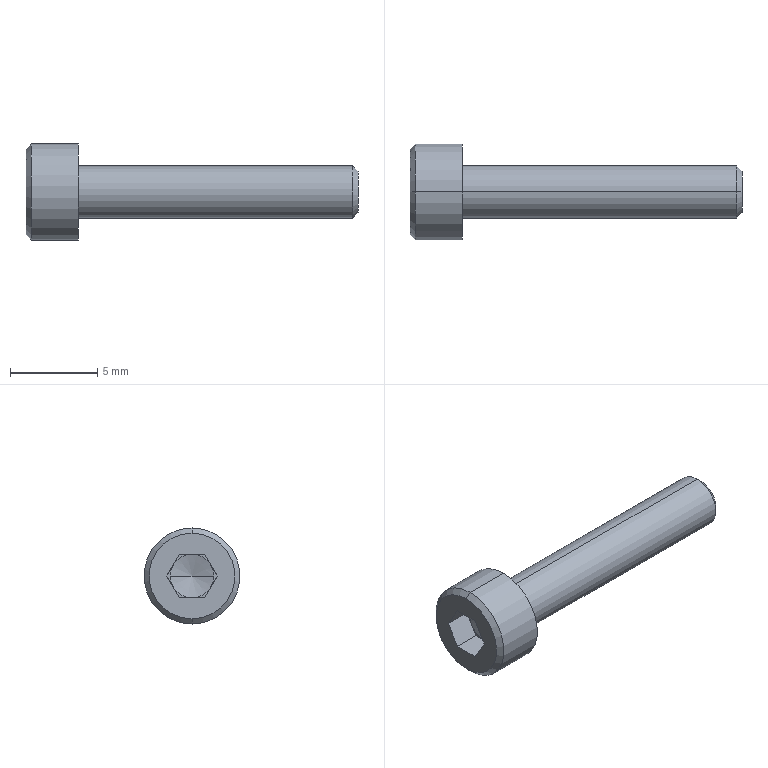Part | STEP file | 0245_302_SCB3-16 | 1 solid | 25 faces | box 19 x 5.5 x 5.5 mm | volume 174.543 mm3 | plane 15 | cone 6 | cylinder 4 | commonest cylinder face diameters 3 x2 5.5 x2